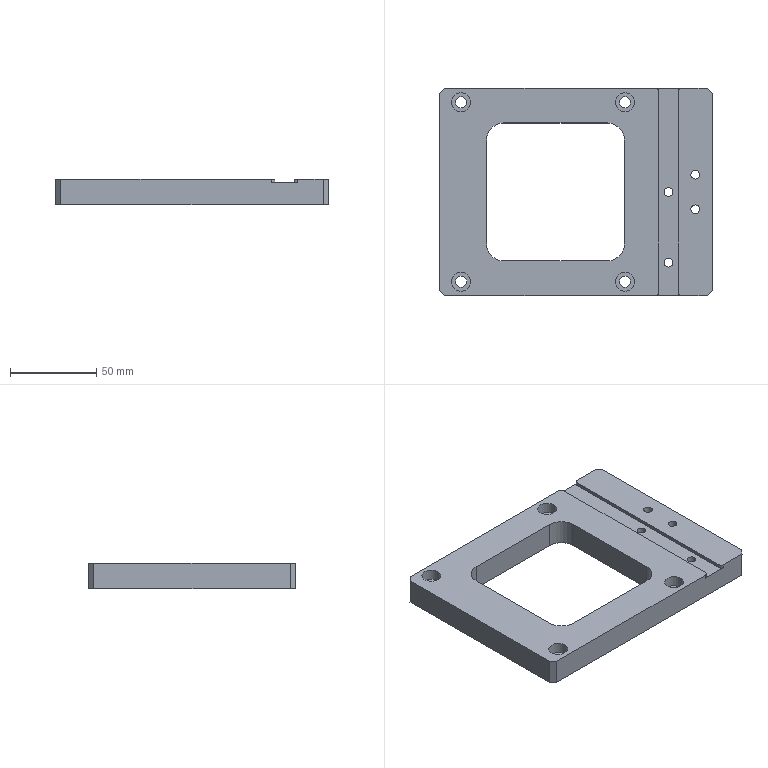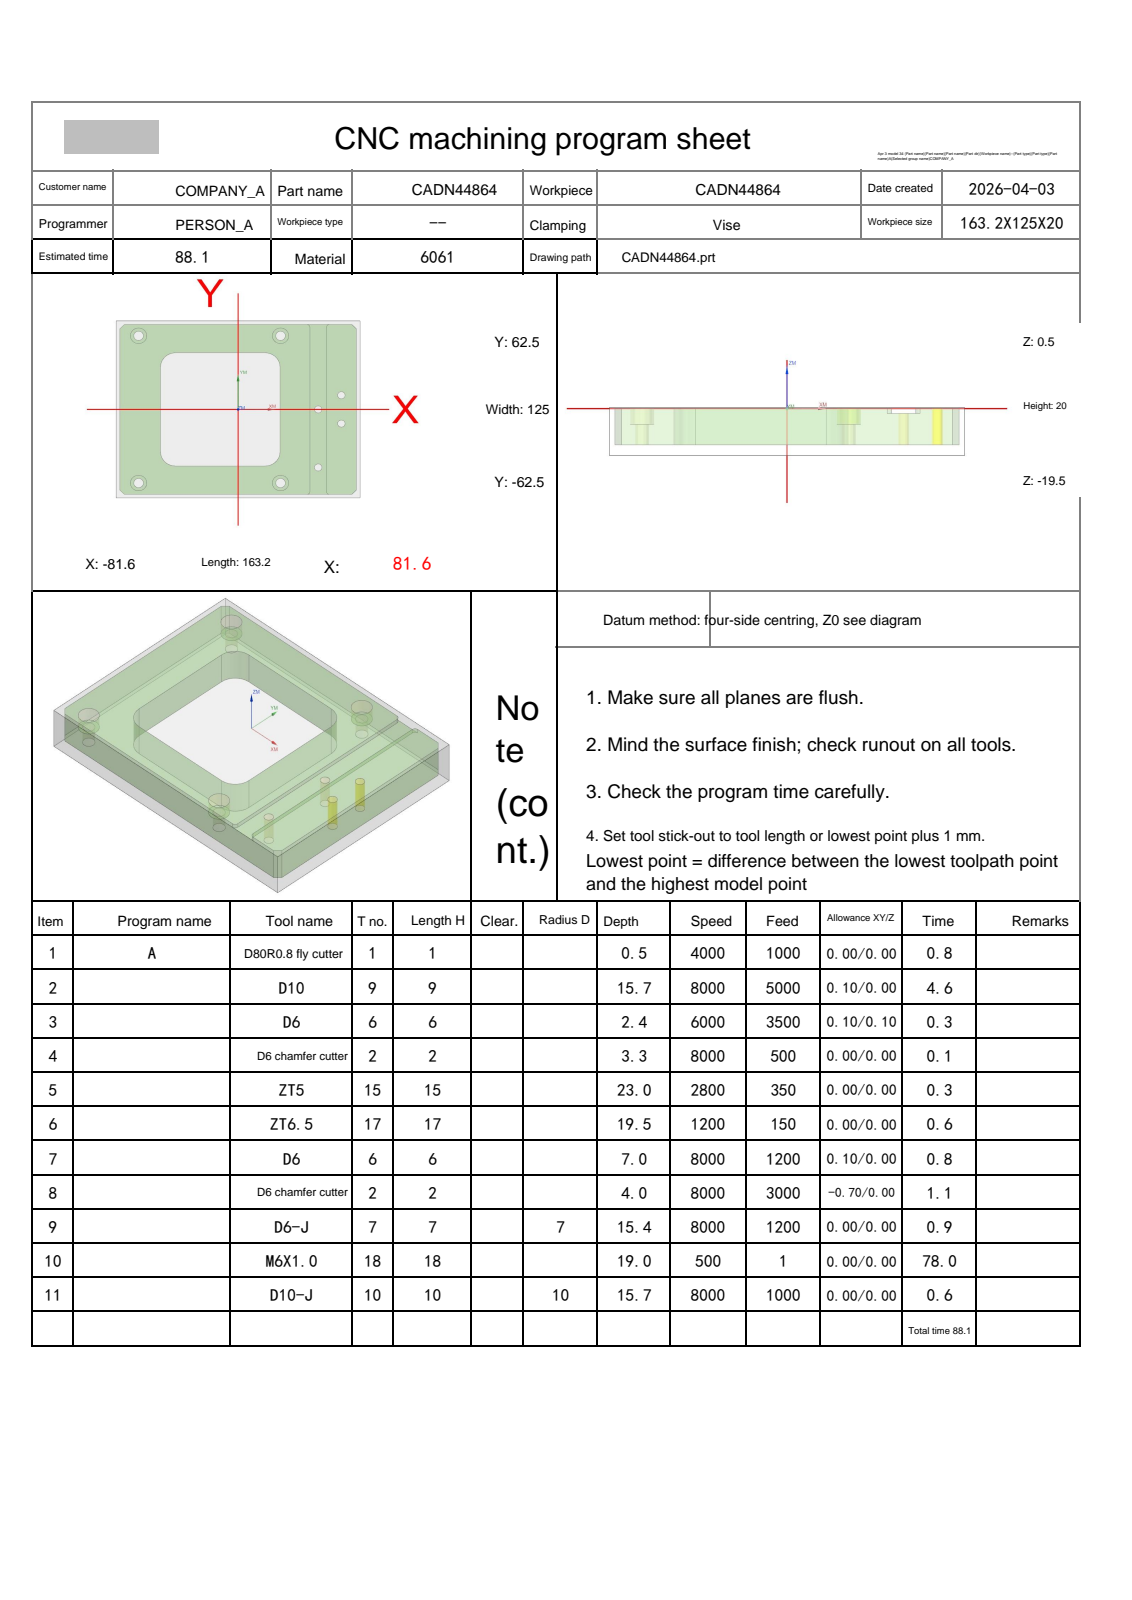NC program | NX | posted by the shop | part box 158.2 x 120 x 15 mm
Lines 1 to 960 of 2334:
%
O0001
(Machine time: 164.34 MIN)
(===Total Tool:9===)
(T1=D80R0.8 fly cutter D=80.  R=0.8  D-  H01 Z=0.    )
(T9=D10     D=10.  R=0.   D-  H09 Z=-15.2 )
(T6=D6      D=6.   R=0.   D-  H06 Z=-6.5  )
(T2=D6 chamfer cutter   D=6.   R=0.   D-  H02 Z=-3.5  )
(T15=ZT5    D=5.   DR_a=118 D-  H15 Z=-22.5 )
(T17=ZT6.5  D=6.5  DR_a=118 D-  H17 Z=-18.95)
(T7=D6-J    D=6.   R=0.   D7  H07 Z=-14.85)
(T18=M6X1.0 D=5.   DR_a=180 D-  H18 Z=-18.5 )
(T10=D10-J  D=10.  R=0.   D10 H10 Z=-15.2 )
G80 G90 G17 G49 G40
G91 G28 Z0
M01
N1 T01 M06
(D80R0.8 fly cutter  D=80. R=0.8 H=01 ce=0.00 di=0.00)
G00 G90 G54 X-124.1 Y50. M03 S4000
G43 H01 Z20.
M08
Z2.
G01 Z0.0 F1000.
X-119.1
X119.1
Y0.0
X-119.1
Y-50.
X119.1
X124.1
Z2.
G00 Z20.
G91 G28 Z0.0
M05
M09
G91 G28 Z0.0
M01
N2 T09 M06
(D10  D=10. R=0. H=09 ce=0.10 di=0.00)
G00 G90 G54 X0.0 Y65.1 M03 S8000
G43 H09 Z20.
M08
Z.5
G01 X76.1 Z.397 F5000.
G02 X79.706 Y63.606 Z.392 I0.0 J-5.1
G01 X82.706 Y60.606 Z.386
G02 X84.2 Y57. Z.381 I-3.606 J-3.606
G01 Y-57. Z.227
G02 X82.706 Y-60.606 Z.221 I-5.1 J0.0
G01 X79.706 Y-63.606 Z.216
G02 X76.1 Y-65.1 Z.21 I-3.606 J3.606
G01 X-76.1 Z.005
G02 X-79.706 Y-63.606 Z-.001 I0.0 J5.1
G01 X-82.706 Y-60.606 Z-.006
G02 X-84.2 Y-57. Z-.012 I3.606 J3.606
G01 Y57. Z-.166
G02 X-82.706 Y60.606 Z-.171 I5.1 J0.0
G01 X-79.706 Y63.606 Z-.177
G02 X-76.1 Y65.1 Z-.182 I3.606 J-3.606
G01 X76.1 Z-.388
G02 X79.706 Y63.606 Z-.393 I0.0 J-5.1
G01 X82.706 Y60.606 Z-.399
G02 X84.2 Y57. Z-.404 I-3.606 J-3.606
G01 Y-57. Z-.558
G02 X82.706 Y-60.606 Z-.564 I-5.1 J0.0
G01 X79.706 Y-63.606 Z-.569
G02 X76.1 Y-65.1 Z-.575 I-3.606 J3.606
G01 X-76.1 Z-.78
G02 X-79.706 Y-63.606 Z-.786 I0.0 J5.1
G01 X-82.706 Y-60.606 Z-.791
G02 X-84.2 Y-57. Z-.797 I3.606 J3.606
G01 Y57. Z-.951
G02 X-82.706 Y60.606 Z-.956 I5.1 J0.0
G01 X-79.706 Y63.606 Z-.962
G02 X-76.1 Y65.1 Z-.967 I3.606 J-3.606
G01 X76.1 Z-1.173
G02 X79.706 Y63.606 Z-1.178 I0.0 J-5.1
G01 X82.706 Y60.606 Z-1.184
G02 X84.2 Y57. Z-1.189 I-3.606 J-3.606
G01 Y-57. Z-1.343
G02 X82.706 Y-60.606 Z-1.349 I-5.1 J0.0
G01 X79.706 Y-63.606 Z-1.354
G02 X76.1 Y-65.1 Z-1.36 I-3.606 J3.606
G01 X-76.1 Z-1.565
G02 X-79.706 Y-63.606 Z-1.571 I0.0 J5.1
G01 X-82.706 Y-60.606 Z-1.576
G02 X-84.2 Y-57. Z-1.582 I3.606 J3.606
G01 Y57. Z-1.736
G02 X-82.706 Y60.606 Z-1.741 I5.1 J0.0
G01 X-79.706 Y63.606 Z-1.747
G02 X-76.1 Y65.1 Z-1.752 I3.606 J-3.606
G01 X76.1 Z-1.958
G02 X79.706 Y63.606 Z-1.963 I0.0 J-5.1
G01 X82.706 Y60.606 Z-1.969
G02 X84.2 Y57. Z-1.974 I-3.606 J-3.606
G01 Y-57. Z-2.128
G02 X82.706 Y-60.606 Z-2.134 I-5.1 J0.0
G01 X79.706 Y-63.606 Z-2.139
G02 X76.1 Y-65.1 Z-2.145 I-3.606 J3.606
G01 X-76.1 Z-2.35
G02 X-79.706 Y-63.606 Z-2.356 I0.0 J5.1
G01 X-82.706 Y-60.606 Z-2.361
G02 X-84.2 Y-57. Z-2.367 I3.606 J3.606
G01 Y57. Z-2.521
G02 X-82.706 Y60.606 Z-2.526 I5.1 J0.0
G01 X-79.706 Y63.606 Z-2.532
G02 X-76.1 Y65.1 Z-2.537 I3.606 J-3.606
G01 X76.1 Z-2.743
G02 X79.706 Y63.606 Z-2.748 I0.0 J-5.1
G01 X82.706 Y60.606 Z-2.754
G02 X84.2 Y57. Z-2.759 I-3.606 J-3.606
G01 Y-57. Z-2.913
G02 X82.706 Y-60.606 Z-2.919 I-5.1 J0.0
G01 X79.706 Y-63.606 Z-2.924
G02 X76.1 Y-65.1 Z-2.93 I-3.606 J3.606
G01 X-76.1 Z-3.135
G02 X-79.706 Y-63.606 Z-3.141 I0.0 J5.1
G01 X-82.706 Y-60.606 Z-3.146
G02 X-84.2 Y-57. Z-3.152 I3.606 J3.606
G01 Y57. Z-3.306
G02 X-82.706 Y60.606 Z-3.311 I5.1 J0.0
G01 X-79.706 Y63.606 Z-3.317
G02 X-76.1 Y65.1 Z-3.322 I3.606 J-3.606
G01 X76.1 Z-3.528
G02 X79.706 Y63.606 Z-3.533 I0.0 J-5.1
G01 X82.706 Y60.606 Z-3.539
G02 X84.2 Y57. Z-3.544 I-3.606 J-3.606
G01 Y-57. Z-3.698
G02 X82.706 Y-60.606 Z-3.704 I-5.1 J0.0
G01 X79.706 Y-63.606 Z-3.709
G02 X76.1 Y-65.1 Z-3.715 I-3.606 J3.606
G01 X-76.1 Z-3.92
G02 X-79.706 Y-63.606 Z-3.926 I0.0 J5.1
G01 X-82.706 Y-60.606 Z-3.931
G02 X-84.2 Y-57. Z-3.937 I3.606 J3.606
G01 Y57. Z-4.091
G02 X-82.706 Y60.606 Z-4.096 I5.1 J0.0
G01 X-79.706 Y63.606 Z-4.102
G02 X-76.1 Y65.1 Z-4.107 I3.606 J-3.606
G01 X76.1 Z-4.313
G02 X79.706 Y63.606 Z-4.318 I0.0 J-5.1
G01 X82.706 Y60.606 Z-4.324
G02 X84.2 Y57. Z-4.329 I-3.606 J-3.606
G01 Y-57. Z-4.483
G02 X82.706 Y-60.606 Z-4.489 I-5.1 J0.0
G01 X79.706 Y-63.606 Z-4.494
G02 X76.1 Y-65.1 Z-4.5 I-3.606 J3.606
G01 X-76.1 Z-4.705
G02 X-79.706 Y-63.606 Z-4.711 I0.0 J5.1
G01 X-82.706 Y-60.606 Z-4.716
G02 X-84.2 Y-57. Z-4.722 I3.606 J3.606
G01 Y57. Z-4.876
G02 X-82.706 Y60.606 Z-4.881 I5.1 J0.0
G01 X-79.706 Y63.606 Z-4.887
G02 X-76.1 Y65.1 Z-4.892 I3.606 J-3.606
G01 X76.1 Z-5.098
G02 X79.706 Y63.606 Z-5.103 I0.0 J-5.1
G01 X82.706 Y60.606 Z-5.109
G02 X84.2 Y57. Z-5.114 I-3.606 J-3.606
G01 Y-57. Z-5.268
G02 X82.706 Y-60.606 Z-5.274 I-5.1 J0.0
G01 X79.706 Y-63.606 Z-5.279
G02 X76.1 Y-65.1 Z-5.285 I-3.606 J3.606
G01 X-76.1 Z-5.49
G02 X-79.706 Y-63.606 Z-5.496 I0.0 J5.1
G01 X-82.706 Y-60.606 Z-5.501
G02 X-84.2 Y-57. Z-5.507 I3.606 J3.606
G01 Y57. Z-5.661
G02 X-82.706 Y60.606 Z-5.666 I5.1 J0.0
G01 X-79.706 Y63.606 Z-5.672
G02 X-76.1 Y65.1 Z-5.677 I3.606 J-3.606
G01 X76.1 Z-5.883
G02 X79.706 Y63.606 Z-5.888 I0.0 J-5.1
G01 X82.706 Y60.606 Z-5.894
G02 X84.2 Y57. Z-5.899 I-3.606 J-3.606
G01 Y-57. Z-6.053
G02 X82.706 Y-60.606 Z-6.059 I-5.1 J0.0
G01 X79.706 Y-63.606 Z-6.064
G02 X76.1 Y-65.1 Z-6.07 I-3.606 J3.606
G01 X-76.1 Z-6.275
G02 X-79.706 Y-63.606 Z-6.281 I0.0 J5.1
G01 X-82.706 Y-60.606 Z-6.286
G02 X-84.2 Y-57. Z-6.292 I3.606 J3.606
G01 Y57. Z-6.446
G02 X-82.706 Y60.606 Z-6.451 I5.1 J0.0
G01 X-79.706 Y63.606 Z-6.457
G02 X-76.1 Y65.1 Z-6.462 I3.606 J-3.606
G01 X76.1 Z-6.668
G02 X79.706 Y63.606 Z-6.673 I0.0 J-5.1
G01 X82.706 Y60.606 Z-6.679
G02 X84.2 Y57. Z-6.684 I-3.606 J-3.606
G01 Y-57. Z-6.838
G02 X82.706 Y-60.606 Z-6.844 I-5.1 J0.0
G01 X79.706 Y-63.606 Z-6.849
G02 X76.1 Y-65.1 Z-6.855 I-3.606 J3.606
G01 X-76.1 Z-7.06
G02 X-79.706 Y-63.606 Z-7.066 I0.0 J5.1
G01 X-82.706 Y-60.606 Z-7.071
G02 X-84.2 Y-57. Z-7.077 I3.606 J3.606
G01 Y57. Z-7.231
G02 X-82.706 Y60.606 Z-7.236 I5.1 J0.0
G01 X-79.706 Y63.606 Z-7.242
G02 X-76.1 Y65.1 Z-7.247 I3.606 J-3.606
G01 X76.1 Z-7.453
G02 X79.706 Y63.606 Z-7.458 I0.0 J-5.1
G01 X82.706 Y60.606 Z-7.464
G02 X84.2 Y57. Z-7.469 I-3.606 J-3.606
G01 Y-57. Z-7.623
G02 X82.706 Y-60.606 Z-7.629 I-5.1 J0.0
G01 X79.706 Y-63.606 Z-7.634
G02 X76.1 Y-65.1 Z-7.64 I-3.606 J3.606
G01 X-76.1 Z-7.845
G02 X-79.706 Y-63.606 Z-7.851 I0.0 J5.1
G01 X-82.706 Y-60.606 Z-7.856
G02 X-84.2 Y-57. Z-7.862 I3.606 J3.606
G01 Y57. Z-8.016
G02 X-82.706 Y60.606 Z-8.021 I5.1 J0.0
G01 X-79.706 Y63.606 Z-8.027
G02 X-76.1 Y65.1 Z-8.032 I3.606 J-3.606
G01 X76.1 Z-8.238
G02 X79.706 Y63.606 Z-8.243 I0.0 J-5.1
G01 X82.706 Y60.606 Z-8.249
G02 X84.2 Y57. Z-8.254 I-3.606 J-3.606
G01 Y-57. Z-8.408
G02 X82.706 Y-60.606 Z-8.414 I-5.1 J0.0
G01 X79.706 Y-63.606 Z-8.419
G02 X76.1 Y-65.1 Z-8.425 I-3.606 J3.606
G01 X-76.1 Z-8.63
G02 X-79.706 Y-63.606 Z-8.636 I0.0 J5.1
G01 X-82.706 Y-60.606 Z-8.641
G02 X-84.2 Y-57. Z-8.647 I3.606 J3.606
G01 Y57. Z-8.801
G02 X-82.706 Y60.606 Z-8.806 I5.1 J0.0
G01 X-79.706 Y63.606 Z-8.812
G02 X-76.1 Y65.1 Z-8.817 I3.606 J-3.606
G01 X76.1 Z-9.023
G02 X79.706 Y63.606 Z-9.028 I0.0 J-5.1
G01 X82.706 Y60.606 Z-9.034
G02 X84.2 Y57. Z-9.039 I-3.606 J-3.606
G01 Y-57. Z-9.193
G02 X82.706 Y-60.606 Z-9.199 I-5.1 J0.0
G01 X79.706 Y-63.606 Z-9.204
G02 X76.1 Y-65.1 Z-9.21 I-3.606 J3.606
G01 X-76.1 Z-9.415
G02 X-79.706 Y-63.606 Z-9.421 I0.0 J5.1
G01 X-82.706 Y-60.606 Z-9.426
G02 X-84.2 Y-57. Z-9.432 I3.606 J3.606
G01 Y57. Z-9.586
G02 X-82.706 Y60.606 Z-9.591 I5.1 J0.0
G01 X-79.706 Y63.606 Z-9.597
G02 X-76.1 Y65.1 Z-9.602 I3.606 J-3.606
G01 X76.1 Z-9.808
G02 X79.706 Y63.606 Z-9.813 I0.0 J-5.1
G01 X82.706 Y60.606 Z-9.819
G02 X84.2 Y57. Z-9.824 I-3.606 J-3.606
G01 Y-57. Z-9.978
G02 X82.706 Y-60.606 Z-9.984 I-5.1 J0.0
G01 X79.706 Y-63.606 Z-9.989
G02 X76.1 Y-65.1 Z-9.995 I-3.606 J3.606
G01 X-76.1 Z-10.2
G02 X-79.706 Y-63.606 Z-10.206 I0.0 J5.1
G01 X-82.706 Y-60.606 Z-10.211
G02 X-84.2 Y-57. Z-10.217 I3.606 J3.606
G01 Y57. Z-10.371
G02 X-82.706 Y60.606 Z-10.376 I5.1 J0.0
G01 X-79.706 Y63.606 Z-10.382
G02 X-76.1 Y65.1 Z-10.387 I3.606 J-3.606
G01 X76.1 Z-10.593
G02 X79.706 Y63.606 Z-10.598 I0.0 J-5.1
G01 X82.706 Y60.606 Z-10.604
G02 X84.2 Y57. Z-10.609 I-3.606 J-3.606
G01 Y-57. Z-10.763
G02 X82.706 Y-60.606 Z-10.769 I-5.1 J0.0
G01 X79.706 Y-63.606 Z-10.774
G02 X76.1 Y-65.1 Z-10.78 I-3.606 J3.606
G01 X-76.1 Z-10.985
G02 X-79.706 Y-63.606 Z-10.991 I0.0 J5.1
G01 X-82.706 Y-60.606 Z-10.996
G02 X-84.2 Y-57. Z-11.002 I3.606 J3.606
G01 Y57. Z-11.156
G02 X-82.706 Y60.606 Z-11.161 I5.1 J0.0
G01 X-79.706 Y63.606 Z-11.167
G02 X-76.1 Y65.1 Z-11.172 I3.606 J-3.606
G01 X76.1 Z-11.378
G02 X79.706 Y63.606 Z-11.383 I0.0 J-5.1
G01 X82.706 Y60.606 Z-11.389
G02 X84.2 Y57. Z-11.394 I-3.606 J-3.606
G01 Y-57. Z-11.548
G02 X82.706 Y-60.606 Z-11.554 I-5.1 J0.0
G01 X79.706 Y-63.606 Z-11.559
G02 X76.1 Y-65.1 Z-11.565 I-3.606 J3.606
G01 X-76.1 Z-11.77
G02 X-79.706 Y-63.606 Z-11.776 I0.0 J5.1
G01 X-82.706 Y-60.606 Z-11.781
G02 X-84.2 Y-57. Z-11.787 I3.606 J3.606
G01 Y57. Z-11.941
G02 X-82.706 Y60.606 Z-11.946 I5.1 J0.0
G01 X-79.706 Y63.606 Z-11.952
G02 X-76.1 Y65.1 Z-11.957 I3.606 J-3.606
G01 X76.1 Z-12.163
G02 X79.706 Y63.606 Z-12.168 I0.0 J-5.1
G01 X82.706 Y60.606 Z-12.174
G02 X84.2 Y57. Z-12.179 I-3.606 J-3.606
G01 Y-57. Z-12.333
G02 X82.706 Y-60.606 Z-12.339 I-5.1 J0.0
G01 X79.706 Y-63.606 Z-12.344
G02 X76.1 Y-65.1 Z-12.35 I-3.606 J3.606
G01 X-76.1 Z-12.555
G02 X-79.706 Y-63.606 Z-12.561 I0.0 J5.1
G01 X-82.706 Y-60.606 Z-12.566
G02 X-84.2 Y-57. Z-12.572 I3.606 J3.606
G01 Y57. Z-12.726
G02 X-82.706 Y60.606 Z-12.731 I5.1 J0.0
G01 X-79.706 Y63.606 Z-12.737
G02 X-76.1 Y65.1 Z-12.742 I3.606 J-3.606
G01 X76.1 Z-12.948
G02 X79.706 Y63.606 Z-12.953 I0.0 J-5.1
G01 X82.706 Y60.606 Z-12.959
G02 X84.2 Y57. Z-12.964 I-3.606 J-3.606
G01 Y-57. Z-13.118
G02 X82.706 Y-60.606 Z-13.124 I-5.1 J0.0
G01 X79.706 Y-63.606 Z-13.129
G02 X76.1 Y-65.1 Z-13.135 I-3.606 J3.606
G01 X-76.1 Z-13.34
G02 X-79.706 Y-63.606 Z-13.346 I0.0 J5.1
G01 X-82.706 Y-60.606 Z-13.351
G02 X-84.2 Y-57. Z-13.357 I3.606 J3.606
G01 Y57. Z-13.511
G02 X-82.706 Y60.606 Z-13.516 I5.1 J0.0
G01 X-79.706 Y63.606 Z-13.522
G02 X-76.1 Y65.1 Z-13.527 I3.606 J-3.606
G01 X76.1 Z-13.733
G02 X79.706 Y63.606 Z-13.738 I0.0 J-5.1
G01 X82.706 Y60.606 Z-13.744
G02 X84.2 Y57. Z-13.749 I-3.606 J-3.606
G01 Y-57. Z-13.903
G02 X82.706 Y-60.606 Z-13.909 I-5.1 J0.0
G01 X79.706 Y-63.606 Z-13.914
G02 X76.1 Y-65.1 Z-13.92 I-3.606 J3.606
G01 X-76.1 Z-14.125
G02 X-79.706 Y-63.606 Z-14.131 I0.0 J5.1
G01 X-82.706 Y-60.606 Z-14.136
G02 X-84.2 Y-57. Z-14.142 I3.606 J3.606
G01 Y57. Z-14.296
G02 X-82.706 Y60.606 Z-14.301 I5.1 J0.0
G01 X-79.706 Y63.606 Z-14.307
G02 X-76.1 Y65.1 Z-14.312 I3.606 J-3.606
G01 X76.1 Z-14.518
G02 X79.706 Y63.606 Z-14.523 I0.0 J-5.1
G01 X82.706 Y60.606 Z-14.529
G02 X84.2 Y57. Z-14.534 I-3.606 J-3.606
G01 Y-57. Z-14.688
G02 X82.706 Y-60.606 Z-14.694 I-5.1 J0.0
G01 X79.706 Y-63.606 Z-14.699
G02 X76.1 Y-65.1 Z-14.705 I-3.606 J3.606
G01 X-76.1 Z-14.91
G02 X-79.706 Y-63.606 Z-14.916 I0.0 J5.1
G01 X-82.706 Y-60.606 Z-14.921
G02 X-84.2 Y-57. Z-14.927 I3.606 J3.606
G01 Y57. Z-15.081
G02 X-82.706 Y60.606 Z-15.086 I5.1 J0.0
G01 X-79.706 Y63.606 Z-15.092
G02 X-76.1 Y65.1 Z-15.097 I3.606 J-3.606
G01 X0.0 Z-15.2
X76.1
G02 X79.706 Y63.606 I0.0 J-5.1
G01 X82.706 Y60.606
G02 X84.2 Y57. I-3.606 J-3.606
G01 Y-57.
G02 X82.706 Y-60.606 I-5.1 J0.0
G01 X79.706 Y-63.606
G02 X76.1 Y-65.1 I-3.606 J3.606
G01 X-76.1
G02 X-79.706 Y-63.606 I0.0 J5.1
G01 X-82.706 Y-60.606
G02 X-84.2 Y-57. I3.606 J3.606
G01 Y57.
G02 X-82.706 Y60.606 I5.1 J0.0
G01 X-79.706 Y63.606
G02 X-76.1 Y65.1 I3.606 J-3.606
G01 X0.0
X.5
Z-14.2
G00 Z20.
G00 G90 X-11.9 Y-34.9 M03 S6000
Z20.
Z.5
G01 X18.1 Z.445 F4000.
G03 X23. Y-30. Z.431 I0.0 J4.9
G01 Y30. Z.321
G03 X22.02 Y32.94 Z.316 I-4.9 J0.0
X18.1 Y34.9 Z.307 I-3.92 J-2.94
G01 X-41.9 Z.198
G03 X-45.82 Y32.94 Z.189 I0.0 J-4.9
X-46.8 Y30. Z.183 I3.92 J-2.94
G01 Y-30. Z.074
G03 X-41.9 Y-34.9 Z.06 I4.9 J0.0
G01 X18.1 Z-.05
G03 X23. Y-30. Z-.064 I0.0 J4.9
G01 Y30. Z-.174
G03 X22.02 Y32.94 Z-.18 I-4.9 J0.0
X18.1 Y34.9 Z-.188 I-3.92 J-2.94
G01 X-41.9 Z-.298
G03 X-45.82 Y32.94 Z-.306 I0.0 J-4.9
X-46.8 Y30. Z-.312 I3.92 J-2.94
G01 Y-30. Z-.421
G03 X-41.9 Y-34.9 Z-.435 I4.9 J0.0
G01 X18.1 Z-.545
G03 X23. Y-30. Z-.559 I0.0 J4.9
G01 Y30. Z-.669
G03 X22.02 Y32.94 Z-.675 I-4.9 J0.0
X18.1 Y34.9 Z-.683 I-3.92 J-2.94
G01 X-41.9 Z-.793
G03 X-45.82 Y32.94 Z-.801 I0.0 J-4.9
X-46.8 Y30. Z-.807 I3.92 J-2.94
G01 Y-30. Z-.917
G03 X-41.9 Y-34.9 Z-.931 I4.9 J0.0
G01 X18.1 Z-1.04
G03 X23. Y-30. Z-1.054 I0.0 J4.9
G01 Y30. Z-1.164
G03 X22.02 Y32.94 Z-1.17 I-4.9 J0.0
X18.1 Y34.9 Z-1.178 I-3.92 J-2.94
G01 X-41.9 Z-1.288
G03 X-45.82 Y32.94 Z-1.296 I0.0 J-4.9
X-46.8 Y30. Z-1.302 I3.92 J-2.94
G01 Y-30. Z-1.412
G03 X-41.9 Y-34.9 Z-1.426 I4.9 J0.0
G01 X18.1 Z-1.535
G03 X23. Y-30. Z-1.55 I0.0 J4.9
G01 Y30. Z-1.659
G03 X22.02 Y32.94 Z-1.665 I-4.9 J0.0
X18.1 Y34.9 Z-1.673 I-3.92 J-2.94
G01 X-41.9 Z-1.783
G03 X-45.82 Y32.94 Z-1.791 I0.0 J-4.9
X-46.8 Y30. Z-1.797 I3.92 J-2.94
G01 Y-30. Z-1.907
G03 X-41.9 Y-34.9 Z-1.921 I4.9 J0.0
G01 X18.1 Z-2.031
G03 X23. Y-30. Z-2.045 I0.0 J4.9
G01 Y30. Z-2.154
G03 X22.02 Y32.94 Z-2.16 I-4.9 J0.0
X18.1 Y34.9 Z-2.169 I-3.92 J-2.94
G01 X-41.9 Z-2.278
G03 X-45.82 Y32.94 Z-2.287 I0.0 J-4.9
X-46.8 Y30. Z-2.292 I3.92 J-2.94
G01 Y-30. Z-2.402
G03 X-41.9 Y-34.9 Z-2.416 I4.9 J0.0
G01 X18.1 Z-2.526
G03 X23. Y-30. Z-2.54 I0.0 J4.9
G01 Y30. Z-2.65
G03 X22.02 Y32.94 Z-2.655 I-4.9 J0.0
X18.1 Y34.9 Z-2.664 I-3.92 J-2.94
G01 X-41.9 Z-2.773
G03 X-45.82 Y32.94 Z-2.782 I0.0 J-4.9
X-46.8 Y30. Z-2.787 I3.92 J-2.94
G01 Y-30. Z-2.897
G03 X-41.9 Y-34.9 Z-2.911 I4.9 J0.0
G01 X18.1 Z-3.021
G03 X23. Y-30. Z-3.035 I0.0 J4.9
G01 Y30. Z-3.145
G03 X22.02 Y32.94 Z-3.151 I-4.9 J0.0
X18.1 Y34.9 Z-3.159 I-3.92 J-2.94
G01 X-41.9 Z-3.269
G03 X-45.82 Y32.94 Z-3.277 I0.0 J-4.9
X-46.8 Y30. Z-3.283 I3.92 J-2.94
G01 Y-30. Z-3.392
G03 X-41.9 Y-34.9 Z-3.406 I4.9 J0.0
G01 X18.1 Z-3.516
G03 X23. Y-30. Z-3.53 I0.0 J4.9
G01 Y30. Z-3.64
G03 X22.02 Y32.94 Z-3.646 I-4.9 J0.0
X18.1 Y34.9 Z-3.654 I-3.92 J-2.94
G01 X-41.9 Z-3.764
G03 X-45.82 Y32.94 Z-3.772 I0.0 J-4.9
X-46.8 Y30. Z-3.778 I3.92 J-2.94
G01 Y-30. Z-3.888
G03 X-41.9 Y-34.9 Z-3.902 I4.9 J0.0
G01 X18.1 Z-4.011
G03 X23. Y-30. Z-4.025 I0.0 J4.9
G01 Y30. Z-4.135
G03 X22.02 Y32.94 Z-4.141 I-4.9 J0.0
X18.1 Y34.9 Z-4.149 I-3.92 J-2.94
G01 X-41.9 Z-4.259
G03 X-45.82 Y32.94 Z-4.267 I0.0 J-4.9
X-46.8 Y30. Z-4.273 I3.92 J-2.94
G01 Y-30. Z-4.383
G03 X-41.9 Y-34.9 Z-4.397 I4.9 J0.0
G01 X18.1 Z-4.506
G03 X23. Y-30. Z-4.521 I0.0 J4.9
G01 Y30. Z-4.63
G03 X22.02 Y32.94 Z-4.636 I-4.9 J0.0
X18.1 Y34.9 Z-4.644 I-3.92 J-2.94
G01 X-41.9 Z-4.754
G03 X-45.82 Y32.94 Z-4.762 I0.0 J-4.9
X-46.8 Y30. Z-4.768 I3.92 J-2.94
G01 Y-30. Z-4.878
G03 X-41.9 Y-34.9 Z-4.892 I4.9 J0.0
G01 X18.1 Z-5.002
G03 X23. Y-30. Z-5.016 I0.0 J4.9
G01 Y30. Z-5.125
G03 X22.02 Y32.94 Z-5.131 I-4.9 J0.0
X18.1 Y34.9 Z-5.139 I-3.92 J-2.94
G01 X-41.9 Z-5.249
G03 X-45.82 Y32.94 Z-5.258 I0.0 J-4.9
X-46.8 Y30. Z-5.263 I3.92 J-2.94
G01 Y-30. Z-5.373
G03 X-41.9 Y-34.9 Z-5.387 I4.9 J0.0
G01 X18.1 Z-5.497
G03 X23. Y-30. Z-5.511 I0.0 J4.9
G01 Y30. Z-5.621
G03 X22.02 Y32.94 Z-5.626 I-4.9 J0.0
X18.1 Y34.9 Z-5.635 I-3.92 J-2.94
G01 X-41.9 Z-5.744
G03 X-45.82 Y32.94 Z-5.753 I0.0 J-4.9
X-46.8 Y30. Z-5.758 I3.92 J-2.94
G01 Y-30. Z-5.868
G03 X-41.9 Y-34.9 Z-5.882 I4.9 J0.0
G01 X18.1 Z-5.992
G03 X23. Y-30. Z-6.006 I0.0 J4.9
G01 Y30. Z-6.116
G03 X22.02 Y32.94 Z-6.122 I-4.9 J0.0
X18.1 Y34.9 Z-6.13 I-3.92 J-2.94
G01 X-41.9 Z-6.24
G03 X-45.82 Y32.94 Z-6.248 I0.0 J-4.9
X-46.8 Y30. Z-6.254 I3.92 J-2.94
G01 Y-30. Z-6.363
G03 X-41.9 Y-34.9 Z-6.377 I4.9 J0.0
G01 X18.1 Z-6.487
G03 X23. Y-30. Z-6.501 I0.0 J4.9
G01 Y30. Z-6.611
G03 X22.02 Y32.94 Z-6.617 I-4.9 J0.0
X18.1 Y34.9 Z-6.625 I-3.92 J-2.94
G01 X-41.9 Z-6.735
G03 X-45.82 Y32.94 Z-6.743 I0.0 J-4.9
X-46.8 Y30. Z-6.749 I3.92 J-2.94
G01 Y-30. Z-6.858
G03 X-41.9 Y-34.9 Z-6.873 I4.9 J0.0
G01 X18.1 Z-6.982
G03 X23. Y-30. Z-6.996 I0.0 J4.9
G01 Y30. Z-7.106
G03 X22.02 Y32.94 Z-7.112 I-4.9 J0.0
X18.1 Y34.9 Z-7.12 I-3.92 J-2.94
G01 X-41.9 Z-7.23
G03 X-45.82 Y32.94 Z-7.238 I0.0 J-4.9
X-46.8 Y30. Z-7.244 I3.92 J-2.94
G01 Y-30. Z-7.354
G03 X-41.9 Y-34.9 Z-7.368 I4.9 J0.0
G01 X18.1 Z-7.477
G03 X23. Y-30. Z-7.492 I0.0 J4.9
G01 Y30. Z-7.601
G03 X22.02 Y32.94 Z-7.607 I-4.9 J0.0
X18.1 Y34.9 Z-7.615 I-3.92 J-2.94
G01 X-41.9 Z-7.725
G03 X-45.82 Y32.94 Z-7.733 I0.0 J-4.9
X-46.8 Y30. Z-7.739 I3.92 J-2.94
G01 Y-30. Z-7.849
G03 X-41.9 Y-34.9 Z-7.863 I4.9 J0.0
G01 X18.1 Z-7.973
G03 X23. Y-30. Z-7.987 I0.0 J4.9
G01 Y30. Z-8.096
G03 X22.02 Y32.94 Z-8.102 I-4.9 J0.0
X18.1 Y34.9 Z-8.11 I-3.92 J-2.94
G01 X-41.9 Z-8.22
G03 X-45.82 Y32.94 Z-8.228 I0.0 J-4.9
X-46.8 Y30. Z-8.234 I3.92 J-2.94
G01 Y-30. Z-8.344
G03 X-41.9 Y-34.9 Z-8.358 I4.9 J0.0
G01 X18.1 Z-8.468
G03 X23. Y-30. Z-8.482 I0.0 J4.9
G01 Y30. Z-8.592
G03 X22.02 Y32.94 Z-8.597 I-4.9 J0.0
X18.1 Y34.9 Z-8.606 I-3.92 J-2.94
G01 X-41.9 Z-8.715
G03 X-45.82 Y32.94 Z-8.724 I0.0 J-4.9
X-46.8 Y30. Z-8.729 I3.92 J-2.94
G01 Y-30. Z-8.839
G03 X-41.9 Y-34.9 Z-8.853 I4.9 J0.0
G01 X18.1 Z-8.963
G03 X23. Y-30. Z-8.977 I0.0 J4.9
G01 Y30. Z-9.087
G03 X22.02 Y32.94 Z-9.092 I-4.9 J0.0
X18.1 Y34.9 Z-9.101 I-3.92 J-2.94
G01 X-41.9 Z-9.21
G03 X-45.82 Y32.94 Z-9.219 I0.0 J-4.9
X-46.8 Y30. Z-9.225 I3.92 J-2.94
G01 Y-30. Z-9.334
G03 X-41.9 Y-34.9 Z-9.348 I4.9 J0.0
G01 X18.1 Z-9.458
G03 X23. Y-30. Z-9.472 I0.0 J4.9
G01 Y30. Z-9.582
G03 X22.02 Y32.94 Z-9.588 I-4.9 J0.0
X18.1 Y34.9 Z-9.596 I-3.92 J-2.94
G01 X-41.9 Z-9.706
G03 X-45.82 Y32.94 Z-9.714 I0.0 J-4.9
X-46.8 Y30. Z-9.72 I3.92 J-2.94
G01 Y-30. Z-9.829
G03 X-41.9 Y-34.9 Z-9.844 I4.9 J0.0
G01 X18.1 Z-9.953
G03 X23. Y-30. Z-9.967 I0.0 J4.9
G01 Y30. Z-10.077
G03 X22.02 Y32.94 Z-10.083 I-4.9 J0.0
X18.1 Y34.9 Z-10.091 I-3.92 J-2.94
G01 X-41.9 Z-10.201
G03 X-45.82 Y32.94 Z-10.209 I0.0 J-4.9
X-46.8 Y30. Z-10.215 I3.92 J-2.94
G01 Y-30. Z-10.325
G03 X-41.9 Y-34.9 Z-10.339 I4.9 J0.0
G01 X18.1 Z-10.448
G03 X23. Y-30. Z-10.462 I0.0 J4.9
G01 Y30. Z-10.572
G03 X22.02 Y32.94 Z-10.578 I-4.9 J0.0
X18.1 Y34.9 Z-10.586 I-3.92 J-2.94
G01 X-41.9 Z-10.696
G03 X-45.82 Y32.94 Z-10.704 I0.0 J-4.9
X-46.8 Y30. Z-10.71 I3.92 J-2.94
G01 Y-30. Z-10.82
G03 X-41.9 Y-34.9 Z-10.834 I4.9 J0.0
G01 X18.1 Z-10.944
G03 X23. Y-30. Z-10.958 I0.0 J4.9
G01 Y30. Z-11.067
G03 X22.02 Y32.94 Z-11.073 I-4.9 J0.0
X18.1 Y34.9 Z-11.081 I-3.92 J-2.94
G01 X-41.9 Z-11.191
G03 X-45.82 Y32.94 Z-11.199 I0.0 J-4.9
X-46.8 Y30. Z-11.205 I3.92 J-2.94
G01 Y-30. Z-11.315
G03 X-41.9 Y-34.9 Z-11.329 I4.9 J0.0
G01 X18.1 Z-11.439
G03 X23. Y-30. Z-11.453 I0.0 J4.9
G01 Y30. Z-11.563
G03 X22.02 Y32.94 Z-11.568 I-4.9 J0.0
X18.1 Y34.9 Z-11.577 I-3.92 J-2.94
G01 X-41.9 Z-11.686
G03 X-45.82 Y32.94 Z-11.695 I0.0 J-4.9
X-46.8 Y30. Z-11.7 I3.92 J-2.94
G01 Y-30. Z-11.81
G03 X-41.9 Y-34.9 Z-11.824 I4.9 J0.0
G01 X18.1 Z-11.934
G03 X23. Y-30. Z-11.948 I0.0 J4.9
G01 Y30. Z-12.058
G03 X22.02 Y32.94 Z-12.063 I-4.9 J0.0
X18.1 Y34.9 Z-12.072 I-3.92 J-2.94
G01 X-41.9 Z-12.181
G03 X-45.82 Y32.94 Z-12.19 I0.0 J-4.9
X-46.8 Y30. Z-12.196 I3.92 J-2.94
G01 Y-30. Z-12.305
G03 X-41.9 Y-34.9 Z-12.319 I4.9 J0.0
G01 X18.1 Z-12.429
G03 X23. Y-30. Z-12.443 I0.0 J4.9
G01 Y30. Z-12.553
G03 X22.02 Y32.94 Z-12.559 I-4.9 J0.0
X18.1 Y34.9 Z-12.567 I-3.92 J-2.94
G01 X-41.9 Z-12.677
G03 X-45.82 Y32.94 Z-12.685 I0.0 J-4.9
X-46.8 Y30. Z-12.691 I3.92 J-2.94
G01 Y-30. Z-12.8
G03 X-41.9 Y-34.9 Z-12.814 I4.9 J0.0
G01 X18.1 Z-12.924
G03 X23. Y-30. Z-12.938 I0.0 J4.9
G01 Y30. Z-13.048
G03 X22.02 Y32.94 Z-13.054 I-4.9 J0.0
X18.1 Y34.9 Z-13.062 I-3.92 J-2.94
G01 X-41.9 Z-13.172
G03 X-45.82 Y32.94 Z-13.18 I0.0 J-4.9
X-46.8 Y30. Z-13.186 I3.92 J-2.94
G01 Y-30. Z-13.296
G03 X-41.9 Y-34.9 Z-13.31 I4.9 J0.0
G01 X18.1 Z-13.419
G03 X23. Y-30. Z-13.433 I0.0 J4.9
G01 Y30. Z-13.543
G03 X22.02 Y32.94 Z-13.549 I-4.9 J0.0
X18.1 Y34.9 Z-13.557 I-3.92 J-2.94
G01 X-41.9 Z-13.667
G03 X-45.82 Y32.94 Z-13.675 I0.0 J-4.9
X-46.8 Y30. Z-13.681 I3.92 J-2.94
G01 Y-30. Z-13.791
G03 X-41.9 Y-34.9 Z-13.805 I4.9 J0.0
G01 X18.1 Z-13.915
G03 X23. Y-30. Z-13.929 I0.0 J4.9
G01 Y30. Z-14.038
G03 X22.02 Y32.94 Z-14.044 I-4.9 J0.0
X18.1 Y34.9 Z-14.052 I-3.92 J-2.94
G01 X-41.9 Z-14.162
G03 X-45.82 Y32.94 Z-14.17 I0.0 J-4.9
X-46.8 Y30. Z-14.176 I3.92 J-2.94
G01 Y-30. Z-14.286
G03 X-41.9 Y-34.9 Z-14.3 I4.9 J0.0
G01 X18.1 Z-14.41
G03 X23. Y-30. Z-14.424 I0.0 J4.9
G01 Y30. Z-14.533
G03 X22.02 Y32.94 Z-14.539 I-4.9 J0.0
X18.1 Y34.9 Z-14.548 I-3.92 J-2.94
G01 X-41.9 Z-14.657
G03 X-45.82 Y32.94 Z-14.666 I0.0 J-4.9
X-46.8 Y30. Z-14.671 I3.92 J-2.94
G01 Y-30. Z-14.781
G03 X-41.9 Y-34.9 Z-14.795 I4.9 J0.0
G01 X-11.9 Z-14.85
X18.1
G03 X23. Y-30. I0.0 J4.9
G01 Y30.
G03 X18.1 Y34.9 I-4.9 J0.0
G01 X-41.9
G03 X-46.8 Y30. I0.0 J-4.9
G01 Y-30.
G03 X-41.9 Y-34.9 I4.9 J0.0
G01 X-11.9
X-11.4
Z-13.85
G00 Z20.
G91 G28 Z0.0
M05
M09
G91 G28 Z0.0
M01
N3 T06 M06
(D6  D=6. R=0. H=06 ce=0.10 di=0.10)
G00 G90 G54 X53.6 Y66. M03 S6000
G43 H06 Z20.
M08
Z.025
G01 Z-.475 F3500.
Y60.6
X50.437
G02 X51.15 Y58. I-4.387 J-2.6
G01 Y-58.
G02 X50.437 Y-60.6 I-5.1 J0.0
G01 X56.763
G02 X56.05 Y-58. I4.387 J2.6
G01 Y58.
G02 X56.763 Y60.6 I5.1 J0.0
G01 X53.6
X53.1
Z.025
G00 Z.5
X53.6 Y66.
Z-.45
G01 Z-.95
Y60.6
X50.437
G02 X51.15 Y58. I-4.387 J-2.6
G01 Y-58.
G02 X50.437 Y-60.6 I-5.1 J0.0
G01 X56.763
G02 X56.05 Y-58. I4.387 J2.6
G01 Y58.
G02 X56.763 Y60.6 I5.1 J0.0
G01 X53.6
X53.1
Z-.45
G00 Z.025
X53.6 Y66.
Z-.925
G01 Z-1.425
Y60.6
X50.437
G02 X51.15 Y58. I-4.387 J-2.6
G01 Y-58.
G02 X50.437 Y-60.6 I-5.1 J0.0
G01 X56.763
G02 X56.05 Y-58. I4.387 J2.6
G01 Y58.
G02 X56.763 Y60.6 I5.1 J0.0
G01 X53.6
X53.1
Z-.925
G00 Z-.45
X53.6 Y66.
Z-1.4
G01 Z-1.9
Y60.6
X50.437
G02 X51.15 Y58. I-4.387 J-2.6
G01 Y-58.
G02 X50.437 Y-60.6 I-5.1 J0.0
G01 X56.763
G02 X56.05 Y-58. I4.387 J2.6
G01 Y58.
G02 X56.763 Y60.6 I5.1 J0.0
G01 X53.6
X53.1
Z-1.4
G00 Z20.
G91 G28 Z0.0
M05
M09
G91 G28 Z0.0
M01
N4 T02 M06
(D6 chamfer cutter  D=6. R=0. H=02 ce=0.00 di=0.10)
G00 G90 G54 X-66.6 Y52. M03 S8000
G43 H02 Z20.
M08
G98 G81 X-66.6 Y52. Z-.8 R1. F500.
X28.4
X69.1 Y10.
X53.6 Y0.0 Z-2.8 R-1.
X69.1 Y-10. Z-.8 R1.
X53.6 Y-41. Z-2.8 R-1.
X28.4 Y-52. Z-.8 R1.
X-66.6
G80
G00 Z20.
G00 G90 X53.6 Y-41. M03 S8000
Z20.
G98 G81 X53.6 Y-41. Z-2.8 R-1. F500.
X69.1 Y-10. Z-.8 R1.
Y10.
X53.6 Y0.0 Z-2.8 R-1.
G80
G00 Z20.
G91 G28 Z0.0
M05
M09
G91 G28 Z0.0
M01
N5 T15 M06
(ZT5 D=5. DR_a=118 H=15)
G00 G90 G54 X53.6 Y-41. M03 S2800
G43 H15 Z20.
M08
G98 G83 X53.6 Y-41. Z-22.502 R-1. F350. Q3.
G98 G83 X69.1 Y-10. Z-22.502 R1. Q3.
Y10.
G98 G83 X53.6 Y0.0 Z-22.502 R-1. Q3.
G80
G00 Z20.
G91 G28 Z0.0
M05
M09
G91 G28 Z0.0
M01
N6 T17 M06
(ZT6.5 D=6.5 DR_a=118 H=17)
G00 G90 G54 X28.4 Y52. M03 S1200
G43 H17 Z20.
M08
G98 G83 X28.4 Y52. Z-18.953 R1. F150. Q2.
X-66.6
Y-52.
X28.4
G80
G00 Z20.
G91 G28 Z0.0
M05
M09
G91 G28 Z0.0
M01
N7 T06 M06
(D6  D=6. R=0. H=06 ce=0.10 di=0.00)
G00 G90 G54 X28.4 Y52. M03 S8000
G43 H06 Z20.
M08
Z.5
G03 X29.6 Y50.8 I1.2 J0.0 F1200.
X30.8 Y52. I0.0 J1.2
X30.8 Y52. Z0.0 I-2.4 J0.0
X30.8 Y52. Z-.5 I-2.4 J0.0
X30.8 Y52. Z-1. I-2.4 J0.0
X30.8 Y52. Z-1.5 I-2.4 J0.0
X30.8 Y52. Z-2. I-2.4 J0.0
X30.8 Y52. Z-2.5 I-2.4 J0.0
X30.8 Y52. Z-3. I-2.4 J0.0
X30.8 Y52. Z-3.5 I-2.4 J0.0
X30.8 Y52. Z-4. I-2.4 J0.0
X30.8 Y52. Z-4.5 I-2.4 J0.0
X30.8 Y52. Z-5. I-2.4 J0.0
X30.8 Y52. Z-5.5 I-2.4 J0.0
X30.8 Y52. Z-6. I-2.4 J0.0
X30.8 Y52. Z-6.5 I-2.4 J0.0
X28.4 Y54.4 I-2.4 J0.0
X26. Y52. I0.0 J-2.4
X28.4 Y49.6 I2.4 J0.0
X30.8 Y52. I0.0 J2.4
X29.6 Y53.2 I-1.2 J0.0
X28.4 Y52. I0.0 J-1.2
G00 Z20.
X-66.6
Z.5
G03 X-65.4 Y50.8 I1.2 J0.0
X-64.2 Y52. I0.0 J1.2
X-64.2 Y52. Z0.0 I-2.4 J0.0
X-64.2 Y52. Z-.5 I-2.4 J0.0
X-64.2 Y52. Z-1. I-2.4 J0.0
X-64.2 Y52. Z-1.5 I-2.4 J0.0
X-64.2 Y52. Z-2. I-2.4 J0.0
X-64.2 Y52. Z-2.5 I-2.4 J0.0
X-64.2 Y52. Z-3. I-2.4 J0.0
X-64.2 Y52. Z-3.5 I-2.4 J0.0
X-64.2 Y52. Z-4. I-2.4 J0.0
X-64.2 Y52. Z-4.5 I-2.4 J0.0
X-64.2 Y52. Z-5. I-2.4 J0.0
X-64.2 Y52. Z-5.5 I-2.4 J0.0
X-64.2 Y52. Z-6. I-2.4 J0.0
X-64.2 Y52. Z-6.5 I-2.4 J0.0
X-66.6 Y54.4 I-2.4 J0.0
X-69. Y52. I0.0 J-2.4
X-66.6 Y49.6 I2.4 J0.0
X-64.2 Y52. I0.0 J2.4
X-65.4 Y53.2 I-1.2 J0.0
X-66.6 Y52. I0.0 J-1.2
G00 Z20.
G00 G90 X28.4 Y-52. M03 S8000
Z20.
Z.5
G03 X29.6 Y-53.2 I1.2 J0.0 F1200.
X30.8 Y-52. I0.0 J1.2
X30.8 Y-52. Z0.0 I-2.4 J0.0
X30.8 Y-52. Z-.5 I-2.4 J0.0
X30.8 Y-52. Z-1. I-2.4 J0.0
X30.8 Y-52. Z-1.5 I-2.4 J0.0
X30.8 Y-52. Z-2. I-2.4 J0.0
X30.8 Y-52. Z-2.5 I-2.4 J0.0
X30.8 Y-52. Z-3. I-2.4 J0.0
X30.8 Y-52. Z-3.5 I-2.4 J0.0
X30.8 Y-52. Z-4. I-2.4 J0.0
X30.8 Y-52. Z-4.5 I-2.4 J0.0
X30.8 Y-52. Z-5. I-2.4 J0.0
X30.8 Y-52. Z-5.5 I-2.4 J0.0
X30.8 Y-52. Z-6. I-2.4 J0.0
X30.8 Y-52. Z-6.5 I-2.4 J0.0
X28.4 Y-49.6 I-2.4 J0.0
X26. Y-52. I0.0 J-2.4
X28.4 Y-54.4 I2.4 J0.0
X30.8 Y-52. I0.0 J2.4
X29.6 Y-50.8 I-1.2 J0.0
X28.4 Y-52. I0.0 J-1.2
G00 Z20.
X-66.6
Z.5
G03 X-65.4 Y-53.2 I1.2 J0.0
X-64.2 Y-52. I0.0 J1.2
X-64.2 Y-52. Z0.0 I-2.4 J0.0
X-64.2 Y-52. Z-.5 I-2.4 J0.0
X-64.2 Y-52. Z-1. I-2.4 J0.0
X-64.2 Y-52. Z-1.5 I-2.4 J0.0
X-64.2 Y-52. Z-2. I-2.4 J0.0
X-64.2 Y-52. Z-2.5 I-2.4 J0.0
X-64.2 Y-52. Z-3. I-2.4 J0.0
X-64.2 Y-52. Z-3.5 I-2.4 J0.0
X-64.2 Y-52. Z-4. I-2.4 J0.0
X-64.2 Y-52. Z-4.5 I-2.4 J0.0
X-64.2 Y-52. Z-5. I-2.4 J0.0
X-64.2 Y-52. Z-5.5 I-2.4 J0.0
X-64.2 Y-52. Z-6. I-2.4 J0.0
X-64.2 Y-52. Z-6.5 I-2.4 J0.0
X-66.6 Y-49.6 I-2.4 J0.0
X-69. Y-52. I0.0 J-2.4
X-66.6 Y-54.4 I2.4 J0.0
X-64.2 Y-52. I0.0 J2.4
X-65.4 Y-50.8 I-1.2 J0.0
X-66.6 Y-52. I0.0 J-1.2
G00 Z20.
G91 G28 Z0.0
M05
M09
G91 G28 Z0.0
M01